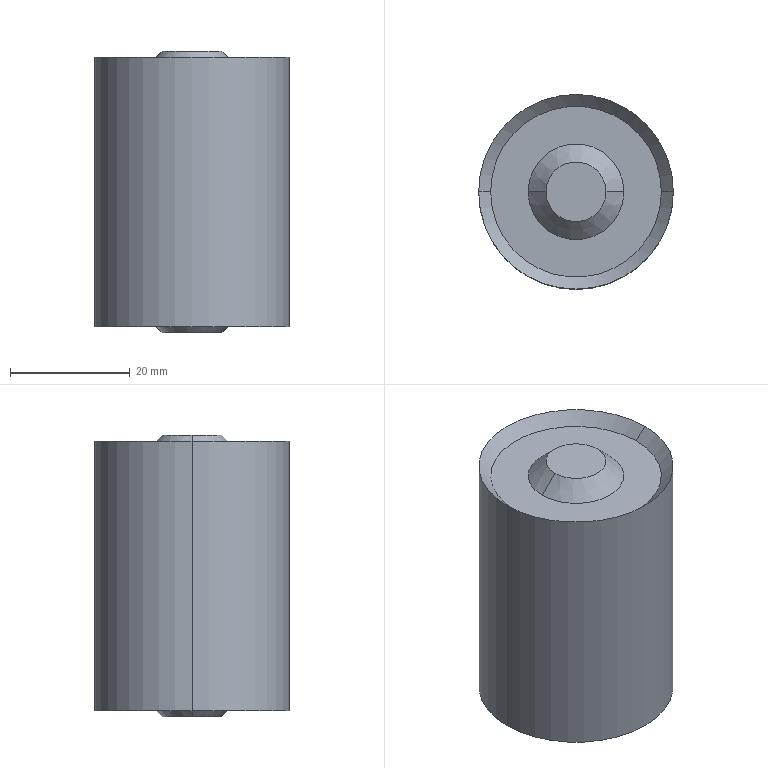Part | SolidWorks | features BaseBody 1 | 1 solid | 14 faces | box 32.5 x 32.5 x 47 mm | volume 35215 mm3 | cone 8 | plane 4 | cylinder 2 | commonest cylinder face diameters 32.5 x2
STEP:
#1=CARTESIAN_POINT('',(-2.25,-59.5,22.5));
#2=VERTEX_POINT('',#1);
#3=CARTESIAN_POINT('',(30.25,-59.5,22.5));
#4=VERTEX_POINT('',#3);
#5=CARTESIAN_POINT('',(14.,-59.5,22.5));
#6=DIRECTION('',(0.,0.,-1.));
#7=DIRECTION('',(-1.,0.,0.));
#8=AXIS2_PLACEMENT_3D('',#5,#6,#7);
#9=CIRCLE('',#8,16.25);
#10=EDGE_CURVE('',#2,#4,#9,.T.);
#11=ORIENTED_EDGE('',*,*,#10,.T.);
#12=CARTESIAN_POINT('',(30.25,-59.5,-22.5));
#13=VERTEX_POINT('',#12);
#14=CARTESIAN_POINT('',(30.25,-59.5,0.));
#15=DIRECTION('',(0.,0.,-1.));
#16=VECTOR('',#15,1000.);
#17=LINE('',#14,#16);
#18=EDGE_CURVE('',#4,#13,#17,.T.);
#19=ORIENTED_EDGE('',*,*,#18,.T.);
#20=CARTESIAN_POINT('',(-2.25,-59.5,-22.5));
#21=VERTEX_POINT('',#20);
#22=CARTESIAN_POINT('',(14.,-59.5,-22.5));
#23=DIRECTION('',(0.,0.,1.));
#24=DIRECTION('',(-1.,0.,0.));
#25=AXIS2_PLACEMENT_3D('',#22,#23,#24);
#26=CIRCLE('',#25,16.25);
#27=EDGE_CURVE('',#13,#21,#26,.T.);
#28=ORIENTED_EDGE('',*,*,#27,.T.);
#29=CARTESIAN_POINT('',(-2.25,-59.5,0.));
#30=DIRECTION('',(0.,0.,-1.));
#31=VECTOR('',#30,1000.);
#32=LINE('',#29,#31);
#33=EDGE_CURVE('',#2,#21,#32,.T.);
#34=ORIENTED_EDGE('',*,*,#33,.F.);
#35=EDGE_LOOP('',(#11,#19,#28,#34));
#36=FACE_OUTER_BOUND('',#35,.T.);
#37=CARTESIAN_POINT('',(14.,-59.5,0.));
#38=DIRECTION('',(0.,0.,-1.));
#39=DIRECTION('',(-1.,0.,0.));
#40=AXIS2_PLACEMENT_3D('',#37,#38,#39);
#41=CYLINDRICAL_SURFACE('',#40,16.25);
#42=ADVANCED_FACE('',(#36),#41,.T.);
#43=CARTESIAN_POINT('',(-0.25,-59.5,20.5));
#44=VERTEX_POINT('',#43);
#45=CARTESIAN_POINT('',(28.25,-59.5,20.5));
#46=VERTEX_POINT('',#45);
#47=CARTESIAN_POINT('',(14.,-59.5,20.5));
#48=DIRECTION('',(0.,0.,1.));
#49=DIRECTION('',(1.,0.,0.));
#50=AXIS2_PLACEMENT_3D('',#47,#48,#49);
#51=CIRCLE('',#50,14.25);
#52=EDGE_CURVE('',#44,#46,#51,.T.);
#53=ORIENTED_EDGE('',*,*,#52,.F.);
#54=CARTESIAN_POINT('',(-2.25,-59.5,22.5));
#55=DIRECTION('',(-0.7071,0.,0.7071));
#56=VECTOR('',#55,1000.);
#57=LINE('',#54,#56);
#58=EDGE_CURVE('',#44,#2,#57,.T.);
#59=ORIENTED_EDGE('',*,*,#58,.T.);
#60=CARTESIAN_POINT('',(14.,-59.5,22.5));
#61=DIRECTION('',(0.,0.,-1.));
#62=DIRECTION('',(-1.,0.,0.));
#63=AXIS2_PLACEMENT_3D('',#60,#61,#62);
#64=CIRCLE('',#63,16.25);
#65=EDGE_CURVE('',#4,#2,#64,.T.);
#66=ORIENTED_EDGE('',*,*,#65,.F.);
#67=CARTESIAN_POINT('',(30.25,-59.5,22.5));
#68=DIRECTION('',(0.7071,0.,0.7071));
#69=VECTOR('',#68,1000.);
#70=LINE('',#67,#69);
#71=EDGE_CURVE('',#46,#4,#70,.T.);
#72=ORIENTED_EDGE('',*,*,#71,.F.);
#73=EDGE_LOOP('',(#53,#59,#66,#72));
#74=FACE_OUTER_BOUND('',#73,.T.);
#75=CARTESIAN_POINT('',(14.,-59.5,22.5));
#76=DIRECTION('',(0.,0.,1.));
#77=DIRECTION('',(1.,0.,0.));
#78=AXIS2_PLACEMENT_3D('',#75,#76,#77);
#79=CONICAL_SURFACE('',#78,16.25,0.7854);
#80=ADVANCED_FACE('',(#74),#79,.F.);
#81=CARTESIAN_POINT('',(28.25,-59.5,-20.5));
#82=VERTEX_POINT('',#81);
#83=CARTESIAN_POINT('',(-0.25,-59.5,-20.5));
#84=VERTEX_POINT('',#83);
#85=CARTESIAN_POINT('',(14.,-59.5,-20.5));
#86=DIRECTION('',(0.,0.,-1.));
#87=DIRECTION('',(-1.,0.,0.));
#88=AXIS2_PLACEMENT_3D('',#85,#86,#87);
#89=CIRCLE('',#88,14.25);
#90=EDGE_CURVE('',#82,#84,#89,.T.);
#91=ORIENTED_EDGE('',*,*,#90,.F.);
#92=CARTESIAN_POINT('',(30.25,-59.5,-22.5));
#93=DIRECTION('',(0.7071,0.,-0.7071));
#94=VECTOR('',#93,1000.);
#95=LINE('',#92,#94);
#96=EDGE_CURVE('',#82,#13,#95,.T.);
#97=ORIENTED_EDGE('',*,*,#96,.T.);
#98=CARTESIAN_POINT('',(14.,-59.5,-22.5));
#99=DIRECTION('',(0.,0.,1.));
#100=DIRECTION('',(-1.,0.,0.));
#101=AXIS2_PLACEMENT_3D('',#98,#99,#100);
#102=CIRCLE('',#101,16.25);
#103=EDGE_CURVE('',#21,#13,#102,.T.);
#104=ORIENTED_EDGE('',*,*,#103,.F.);
#105=CARTESIAN_POINT('',(-2.25,-59.5,-22.5));
#106=DIRECTION('',(-0.7071,0.,-0.7071));
#107=VECTOR('',#106,1000.);
#108=LINE('',#105,#107);
#109=EDGE_CURVE('',#84,#21,#108,.T.);
#110=ORIENTED_EDGE('',*,*,#109,.F.);
#111=EDGE_LOOP('',(#91,#97,#104,#110));
#112=FACE_OUTER_BOUND('',#111,.T.);
#113=CARTESIAN_POINT('',(14.,-59.5,-22.5));
#114=DIRECTION('',(0.,0.,-1.));
#115=DIRECTION('',(-1.,0.,0.));
#116=AXIS2_PLACEMENT_3D('',#113,#114,#115);
#117=CONICAL_SURFACE('',#116,16.25,0.7854);
#118=ADVANCED_FACE('',(#112),#117,.F.);
#119=CARTESIAN_POINT('',(9.,-59.5,23.5));
#120=VERTEX_POINT('',#119);
#121=CARTESIAN_POINT('',(19.,-59.5,23.5));
#122=VERTEX_POINT('',#121);
#123=CARTESIAN_POINT('',(14.,-59.5,23.5));
#124=DIRECTION('',(0.,0.,-1.));
#125=DIRECTION('',(-1.,0.,0.));
#126=AXIS2_PLACEMENT_3D('',#123,#124,#125);
#127=CIRCLE('',#126,5.);
#128=EDGE_CURVE('',#120,#122,#127,.T.);
#129=ORIENTED_EDGE('',*,*,#128,.T.);
#130=CARTESIAN_POINT('',(22.,-59.5,20.5));
#131=VERTEX_POINT('',#130);
#132=CARTESIAN_POINT('',(22.,-59.5,20.5));
#133=DIRECTION('',(0.7071,0.,-0.7071));
#134=VECTOR('',#133,1000.);
#135=LINE('',#132,#134);
#136=EDGE_CURVE('',#122,#131,#135,.T.);
#137=ORIENTED_EDGE('',*,*,#136,.T.);
#138=CARTESIAN_POINT('',(6.,-59.5,20.5));
#139=VERTEX_POINT('',#138);
#140=CARTESIAN_POINT('',(14.,-59.5,20.5));
#141=DIRECTION('',(0.,0.,-1.));
#142=DIRECTION('',(-1.,0.,0.));
#143=AXIS2_PLACEMENT_3D('',#140,#141,#142);
#144=CIRCLE('',#143,8.);
#145=EDGE_CURVE('',#139,#131,#144,.T.);
#146=ORIENTED_EDGE('',*,*,#145,.F.);
#147=CARTESIAN_POINT('',(6.,-59.5,20.5));
#148=DIRECTION('',(-0.7071,0.,-0.7071));
#149=VECTOR('',#148,1000.);
#150=LINE('',#147,#149);
#151=EDGE_CURVE('',#120,#139,#150,.T.);
#152=ORIENTED_EDGE('',*,*,#151,.F.);
#153=EDGE_LOOP('',(#129,#137,#146,#152));
#154=FACE_OUTER_BOUND('',#153,.T.);
#155=CARTESIAN_POINT('',(14.,-59.5,20.5));
#156=DIRECTION('',(0.,0.,-1.));
#157=DIRECTION('',(-1.,0.,0.));
#158=AXIS2_PLACEMENT_3D('',#155,#156,#157);
#159=CONICAL_SURFACE('',#158,8.,0.7854);
#160=ADVANCED_FACE('',(#154),#159,.T.);
#161=CARTESIAN_POINT('',(19.,-59.5,-23.5));
#162=VERTEX_POINT('',#161);
#163=CARTESIAN_POINT('',(9.,-59.5,-23.5));
#164=VERTEX_POINT('',#163);
#165=CARTESIAN_POINT('',(14.,-59.5,-23.5));
#166=DIRECTION('',(0.,0.,1.));
#167=DIRECTION('',(1.,0.,0.));
#168=AXIS2_PLACEMENT_3D('',#165,#166,#167);
#169=CIRCLE('',#168,5.);
#170=EDGE_CURVE('',#162,#164,#169,.T.);
#171=ORIENTED_EDGE('',*,*,#170,.T.);
#172=CARTESIAN_POINT('',(6.,-59.5,-20.5));
#173=VERTEX_POINT('',#172);
#174=CARTESIAN_POINT('',(6.,-59.5,-20.5));
#175=DIRECTION('',(-0.7071,0.,0.7071));
#176=VECTOR('',#175,1000.);
#177=LINE('',#174,#176);
#178=EDGE_CURVE('',#164,#173,#177,.T.);
#179=ORIENTED_EDGE('',*,*,#178,.T.);
#180=CARTESIAN_POINT('',(22.,-59.5,-20.5));
#181=VERTEX_POINT('',#180);
#182=CARTESIAN_POINT('',(14.,-59.5,-20.5));
#183=DIRECTION('',(0.,0.,1.));
#184=DIRECTION('',(1.,0.,0.));
#185=AXIS2_PLACEMENT_3D('',#182,#183,#184);
#186=CIRCLE('',#185,8.);
#187=EDGE_CURVE('',#181,#173,#186,.T.);
#188=ORIENTED_EDGE('',*,*,#187,.F.);
#189=CARTESIAN_POINT('',(22.,-59.5,-20.5));
#190=DIRECTION('',(0.7071,0.,0.7071));
#191=VECTOR('',#190,1000.);
#192=LINE('',#189,#191);
#193=EDGE_CURVE('',#162,#181,#192,.T.);
#194=ORIENTED_EDGE('',*,*,#193,.F.);
#195=EDGE_LOOP('',(#171,#179,#188,#194));
#196=FACE_OUTER_BOUND('',#195,.T.);
#197=CARTESIAN_POINT('',(14.,-59.5,-20.5));
#198=DIRECTION('',(0.,0.,1.));
#199=DIRECTION('',(1.,0.,0.));
#200=AXIS2_PLACEMENT_3D('',#197,#198,#199);
#201=CONICAL_SURFACE('',#200,8.,0.7854);
#202=ADVANCED_FACE('',(#196),#201,.T.);
#203=ORIENTED_EDGE('',*,*,#170,.F.);
#204=CARTESIAN_POINT('',(14.,-59.5,-23.5));
#205=DIRECTION('',(0.,0.,1.));
#206=DIRECTION('',(1.,0.,0.));
#207=AXIS2_PLACEMENT_3D('',#204,#205,#206);
#208=CIRCLE('',#207,5.);
#209=EDGE_CURVE('',#164,#162,#208,.T.);
#210=ORIENTED_EDGE('',*,*,#209,.F.);
#211=EDGE_LOOP('',(#203,#210));
#212=FACE_OUTER_BOUND('',#211,.T.);
#213=CARTESIAN_POINT('',(14.,-62.,-23.5));
#214=DIRECTION('',(0.,0.,-1.));
#215=DIRECTION('',(0.,-1.,0.));
#216=AXIS2_PLACEMENT_3D('',#213,#214,#215);
#217=PLANE('',#216);
#218=ADVANCED_FACE('',(#212),#217,.T.);
#219=ORIENTED_EDGE('',*,*,#128,.F.);
#220=CARTESIAN_POINT('',(14.,-59.5,23.5));
#221=DIRECTION('',(0.,0.,-1.));
#222=DIRECTION('',(-1.,0.,0.));
#223=AXIS2_PLACEMENT_3D('',#220,#221,#222);
#224=CIRCLE('',#223,5.);
#225=EDGE_CURVE('',#122,#120,#224,.T.);
#226=ORIENTED_EDGE('',*,*,#225,.F.);
#227=EDGE_LOOP('',(#219,#226));
#228=FACE_OUTER_BOUND('',#227,.T.);
#229=CARTESIAN_POINT('',(14.,-62.,23.5));
#230=DIRECTION('',(0.,0.,1.));
#231=DIRECTION('',(1.,0.,0.));
#232=AXIS2_PLACEMENT_3D('',#229,#230,#231);
#233=PLANE('',#232);
#234=ADVANCED_FACE('',(#228),#233,.T.);
#235=ORIENTED_EDGE('',*,*,#187,.T.);
#236=CARTESIAN_POINT('',(14.,-59.5,-20.5));
#237=DIRECTION('',(0.,0.,1.));
#238=DIRECTION('',(1.,0.,0.));
#239=AXIS2_PLACEMENT_3D('',#236,#237,#238);
#240=CIRCLE('',#239,8.);
#241=EDGE_CURVE('',#173,#181,#240,.T.);
#242=ORIENTED_EDGE('',*,*,#241,.T.);
#243=EDGE_LOOP('',(#235,#242));
#244=FACE_BOUND('',#243,.T.);
#245=CARTESIAN_POINT('',(14.,-59.5,-20.5));
#246=DIRECTION('',(0.,0.,-1.));
#247=DIRECTION('',(-1.,0.,0.));
#248=AXIS2_PLACEMENT_3D('',#245,#246,#247);
#249=CIRCLE('',#248,14.25);
#250=EDGE_CURVE('',#84,#82,#249,.T.);
#251=ORIENTED_EDGE('',*,*,#250,.T.);
#252=ORIENTED_EDGE('',*,*,#90,.T.);
#253=EDGE_LOOP('',(#251,#252));
#254=FACE_OUTER_BOUND('',#253,.T.);
#255=CARTESIAN_POINT('',(14.,-70.625,-20.5));
#256=DIRECTION('',(0.,0.,-1.));
#257=DIRECTION('',(0.,-1.,0.));
#258=AXIS2_PLACEMENT_3D('',#255,#256,#257);
#259=PLANE('',#258);
#260=ADVANCED_FACE('',(#244,#254),#259,.T.);
#261=ORIENTED_EDGE('',*,*,#145,.T.);
#262=CARTESIAN_POINT('',(14.,-59.5,20.5));
#263=DIRECTION('',(0.,0.,-1.));
#264=DIRECTION('',(-1.,0.,0.));
#265=AXIS2_PLACEMENT_3D('',#262,#263,#264);
#266=CIRCLE('',#265,8.);
#267=EDGE_CURVE('',#131,#139,#266,.T.);
#268=ORIENTED_EDGE('',*,*,#267,.T.);
#269=EDGE_LOOP('',(#261,#268));
#270=FACE_BOUND('',#269,.T.);
#271=CARTESIAN_POINT('',(14.,-59.5,20.5));
#272=DIRECTION('',(0.,0.,1.));
#273=DIRECTION('',(1.,0.,0.));
#274=AXIS2_PLACEMENT_3D('',#271,#272,#273);
#275=CIRCLE('',#274,14.25);
#276=EDGE_CURVE('',#46,#44,#275,.T.);
#277=ORIENTED_EDGE('',*,*,#276,.T.);
#278=ORIENTED_EDGE('',*,*,#52,.T.);
#279=EDGE_LOOP('',(#277,#278));
#280=FACE_OUTER_BOUND('',#279,.T.);
#281=CARTESIAN_POINT('',(14.,-70.625,20.5));
#282=DIRECTION('',(0.,0.,1.));
#283=DIRECTION('',(1.,0.,0.));
#284=AXIS2_PLACEMENT_3D('',#281,#282,#283);
#285=PLANE('',#284);
#286=ADVANCED_FACE('',(#270,#280),#285,.T.);
#287=ORIENTED_EDGE('',*,*,#178,.F.);
#288=ORIENTED_EDGE('',*,*,#209,.T.);
#289=ORIENTED_EDGE('',*,*,#193,.T.);
#290=ORIENTED_EDGE('',*,*,#241,.F.);
#291=EDGE_LOOP('',(#287,#288,#289,#290));
#292=FACE_OUTER_BOUND('',#291,.T.);
#293=CARTESIAN_POINT('',(14.,-59.5,-20.5));
#294=DIRECTION('',(0.,0.,1.));
#295=DIRECTION('',(1.,0.,0.));
#296=AXIS2_PLACEMENT_3D('',#293,#294,#295);
#297=CONICAL_SURFACE('',#296,8.,0.7854);
#298=ADVANCED_FACE('',(#292),#297,.T.);
#299=ORIENTED_EDGE('',*,*,#136,.F.);
#300=ORIENTED_EDGE('',*,*,#225,.T.);
#301=ORIENTED_EDGE('',*,*,#151,.T.);
#302=ORIENTED_EDGE('',*,*,#267,.F.);
#303=EDGE_LOOP('',(#299,#300,#301,#302));
#304=FACE_OUTER_BOUND('',#303,.T.);
#305=CARTESIAN_POINT('',(14.,-59.5,20.5));
#306=DIRECTION('',(0.,0.,-1.));
#307=DIRECTION('',(-1.,0.,0.));
#308=AXIS2_PLACEMENT_3D('',#305,#306,#307);
#309=CONICAL_SURFACE('',#308,8.,0.7854);
#310=ADVANCED_FACE('',(#304),#309,.T.);
#311=ORIENTED_EDGE('',*,*,#96,.F.);
#312=ORIENTED_EDGE('',*,*,#250,.F.);
#313=ORIENTED_EDGE('',*,*,#109,.T.);
#314=ORIENTED_EDGE('',*,*,#27,.F.);
#315=EDGE_LOOP('',(#311,#312,#313,#314));
#316=FACE_OUTER_BOUND('',#315,.T.);
#317=CARTESIAN_POINT('',(14.,-59.5,-22.5));
#318=DIRECTION('',(0.,0.,-1.));
#319=DIRECTION('',(-1.,0.,0.));
#320=AXIS2_PLACEMENT_3D('',#317,#318,#319);
#321=CONICAL_SURFACE('',#320,16.25,0.7854);
#322=ADVANCED_FACE('',(#316),#321,.F.);
#323=ORIENTED_EDGE('',*,*,#58,.F.);
#324=ORIENTED_EDGE('',*,*,#276,.F.);
#325=ORIENTED_EDGE('',*,*,#71,.T.);
#326=ORIENTED_EDGE('',*,*,#10,.F.);
#327=EDGE_LOOP('',(#323,#324,#325,#326));
#328=FACE_OUTER_BOUND('',#327,.T.);
#329=CARTESIAN_POINT('',(14.,-59.5,22.5));
#330=DIRECTION('',(0.,0.,1.));
#331=DIRECTION('',(1.,0.,0.));
#332=AXIS2_PLACEMENT_3D('',#329,#330,#331);
#333=CONICAL_SURFACE('',#332,16.25,0.7854);
#334=ADVANCED_FACE('',(#328),#333,.F.);
#335=ORIENTED_EDGE('',*,*,#18,.F.);
#336=ORIENTED_EDGE('',*,*,#65,.T.);
#337=ORIENTED_EDGE('',*,*,#33,.T.);
#338=ORIENTED_EDGE('',*,*,#103,.T.);
#339=EDGE_LOOP('',(#335,#336,#337,#338));
#340=FACE_OUTER_BOUND('',#339,.T.);
#341=CARTESIAN_POINT('',(14.,-59.5,0.));
#342=DIRECTION('',(0.,0.,-1.));
#343=DIRECTION('',(-1.,0.,0.));
#344=AXIS2_PLACEMENT_3D('',#341,#342,#343);
#345=CYLINDRICAL_SURFACE('',#344,16.25);
#346=ADVANCED_FACE('',(#340),#345,.T.);
#347=CLOSED_SHELL('',(#42,#80,#118,#160,#202,#218,#234,#260,#286,#298,#310,#322,#334,#346));
#348=MANIFOLD_SOLID_BREP('',#347);
#349=CARTESIAN_POINT('',(0.,0.,0.));
#350=DIRECTION('',(0.,0.,1.));
#351=DIRECTION('',(1.,0.,0.));
#352=AXIS2_PLACEMENT_3D('',#349,#350,#351);
#353=(LENGTH_UNIT()NAMED_UNIT(*)SI_UNIT(.MILLI.,.METRE.));
#354=UNCERTAINTY_MEASURE_WITH_UNIT(LENGTH_MEASURE(0.00001),#353,'','');
#355=(NAMED_UNIT(*)PLANE_ANGLE_UNIT()SI_UNIT($,.RADIAN.));
#356=(NAMED_UNIT(*)SI_UNIT($,.STERADIAN.)SOLID_ANGLE_UNIT());
#357=(GEOMETRIC_REPRESENTATION_CONTEXT(3)GLOBAL_UNCERTAINTY_ASSIGNED_CONTEXT((#354))GLOBAL_UNIT_ASSIGNED_CONTEXT((#353,#355,#356))REPRESENTATION_CONTEXT('',''));
#358=ADVANCED_BREP_SHAPE_REPRESENTATION('',(#348,#352),#357);